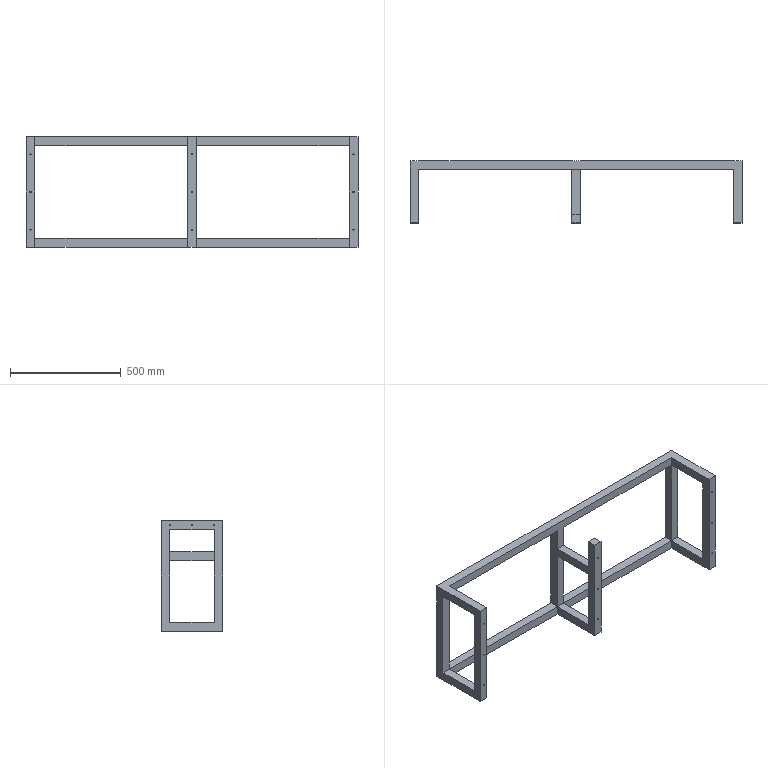Part | STEP file | 1 solid | 147 faces | box 1500 x 280 x 500 mm | volume 11121240 mm3 | cylinder 68 | plane 47 | cone 32 | commonest cylinder face diameters 5.5 x18 10 x18 5 x16 3.3 x12 4.2 x4